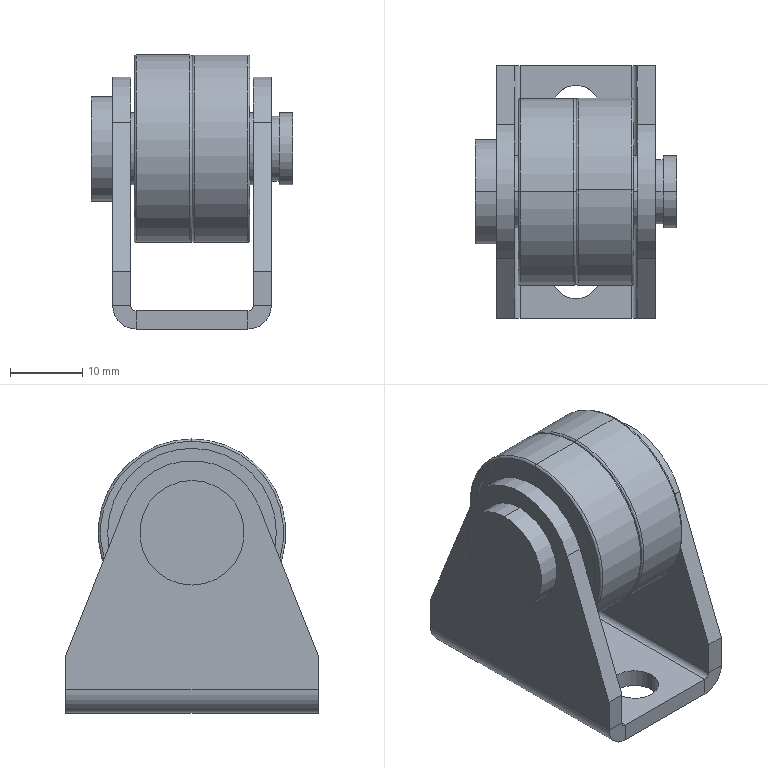Part | NX | features BREP 3 | 4 solids | 371 faces | box 28 x 35 x 38 mm | volume 12259 mm3 | sphere 168 | cylinder 70 | plane 69 | torus 64 | commonest cylinder face diameters 23.4 x16 10 x12 14.9 x8 16.471 x8 6.6 x4 17.84 x4